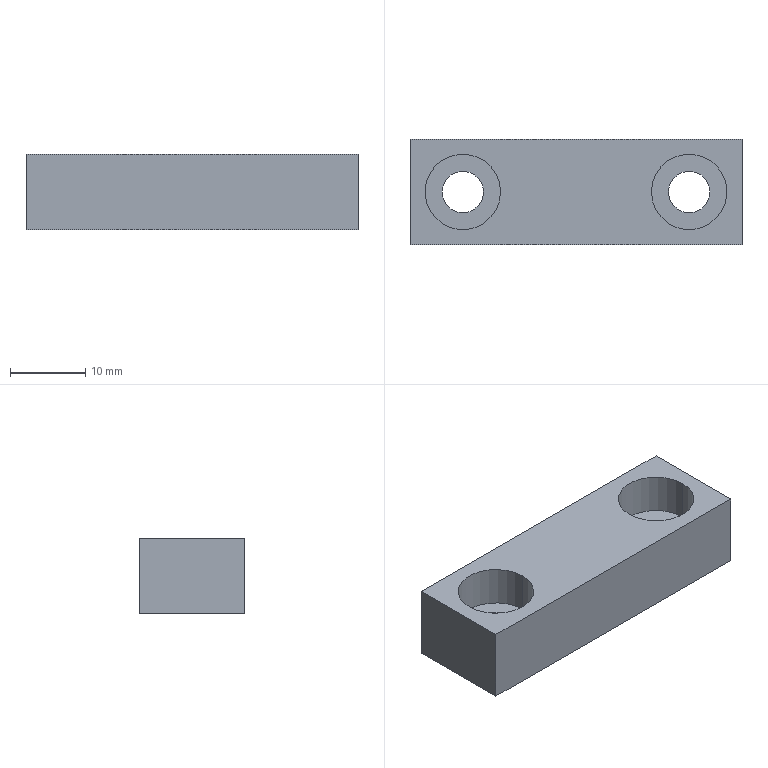Part | STEP file | PN_0061 (stop block) | 1 solid | 16 faces | box 44 x 14 x 10 mm | volume 5093 mm3 | cylinder 8 | plane 8 | commonest cylinder face diameters 5.5 x4 10 x4
STEP:
#1=CARTESIAN_POINT('',(0.,0.,0.));
#2=DIRECTION('',(0.,0.,1.));
#3=DIRECTION('',(1.,0.,0.));
#4=AXIS2_PLACEMENT_3D('',#1,#2,#3);
#5=CARTESIAN_POINT('',(-10.,0.,4.6));
#6=VERTEX_POINT('',#5);
#7=CARTESIAN_POINT('',(-10.,0.,10.));
#8=VERTEX_POINT('',#7);
#9=CARTESIAN_POINT('',(-10.,0.,10.));
#10=DIRECTION('',(0.,0.,1.));
#11=VECTOR('',#10,1.);
#12=LINE('',#9,#11);
#13=CARTESIAN_POINT('',(-15.,0.,10.));
#14=DIRECTION('',(0.,0.,1.));
#15=DIRECTION('',(1.,0.,0.));
#16=AXIS2_PLACEMENT_3D('',#13,#14,#15);
#17=CYLINDRICAL_SURFACE('',#16,5.);
#18=CARTESIAN_POINT('',(6.283,0.));
#19=DIRECTION('',(0.,1.));
#20=VECTOR('',#19,1.);
#21=LINE('',#18,#20);
#22=(GEOMETRIC_REPRESENTATION_CONTEXT(2)PARAMETRIC_REPRESENTATION_CONTEXT()REPRESENTATION_CONTEXT('',''));
#23=DEFINITIONAL_REPRESENTATION('',(#21),#22);
#24=PCURVE('',#17,#23);
#25=CARTESIAN_POINT('',(-15.,0.,10.));
#26=DIRECTION('',(0.,0.,1.));
#27=DIRECTION('',(1.,0.,0.));
#28=AXIS2_PLACEMENT_3D('',#25,#26,#27);
#29=CYLINDRICAL_SURFACE('',#28,5.);
#30=CARTESIAN_POINT('',(0.,0.));
#31=DIRECTION('',(0.,1.));
#32=VECTOR('',#31,1.);
#33=LINE('',#30,#32);
#34=(GEOMETRIC_REPRESENTATION_CONTEXT(2)PARAMETRIC_REPRESENTATION_CONTEXT()REPRESENTATION_CONTEXT('',''));
#35=DEFINITIONAL_REPRESENTATION('',(#33),#34);
#36=PCURVE('',#29,#35);
#37=SURFACE_CURVE('',#12,(#24,#36),.PCURVE_S1.);
#38=EDGE_CURVE('',#6,#8,#37,.T.);
#39=ORIENTED_EDGE('',*,*,#38,.T.);
#40=CARTESIAN_POINT('',(-20.,0.,10.));
#41=VERTEX_POINT('',#40);
#42=CARTESIAN_POINT('',(-15.,0.,10.));
#43=DIRECTION('',(0.,0.,1.));
#44=DIRECTION('',(1.,0.,0.));
#45=AXIS2_PLACEMENT_3D('',#42,#43,#44);
#46=CIRCLE('',#45,5.);
#47=CARTESIAN_POINT('',(0.,0.));
#48=DIRECTION('',(1.,0.));
#49=VECTOR('',#48,1.);
#50=LINE('',#47,#49);
#51=(GEOMETRIC_REPRESENTATION_CONTEXT(2)PARAMETRIC_REPRESENTATION_CONTEXT()REPRESENTATION_CONTEXT('',''));
#52=DEFINITIONAL_REPRESENTATION('',(#50),#51);
#53=PCURVE('',#17,#52);
#54=CARTESIAN_POINT('',(0.,0.,10.));
#55=DIRECTION('',(0.,0.,1.));
#56=DIRECTION('',(1.,0.,0.));
#57=AXIS2_PLACEMENT_3D('',#54,#55,#56);
#58=PLANE('',#57);
#59=CARTESIAN_POINT('',(-15.,0.));
#60=DIRECTION('',(1.,0.));
#61=AXIS2_PLACEMENT_2D('',#59,#60);
#62=CIRCLE('',#61,5.);
#63=(GEOMETRIC_REPRESENTATION_CONTEXT(2)PARAMETRIC_REPRESENTATION_CONTEXT()REPRESENTATION_CONTEXT('',''));
#64=DEFINITIONAL_REPRESENTATION('',(#62),#63);
#65=PCURVE('',#58,#64);
#66=SURFACE_CURVE('',#46,(#53,#65),.PCURVE_S1.);
#67=EDGE_CURVE('',#41,#8,#66,.T.);
#68=ORIENTED_EDGE('',*,*,#67,.F.);
#69=CARTESIAN_POINT('',(-20.,0.,4.6));
#70=VERTEX_POINT('',#69);
#71=CARTESIAN_POINT('',(-20.,0.,10.));
#72=DIRECTION('',(0.,0.,1.));
#73=VECTOR('',#72,1.);
#74=LINE('',#71,#73);
#75=CARTESIAN_POINT('',(3.142,0.));
#76=DIRECTION('',(0.,1.));
#77=VECTOR('',#76,1.);
#78=LINE('',#75,#77);
#79=(GEOMETRIC_REPRESENTATION_CONTEXT(2)PARAMETRIC_REPRESENTATION_CONTEXT()REPRESENTATION_CONTEXT('',''));
#80=DEFINITIONAL_REPRESENTATION('',(#78),#79);
#81=PCURVE('',#17,#80);
#82=CARTESIAN_POINT('',(3.142,0.));
#83=DIRECTION('',(0.,1.));
#84=VECTOR('',#83,1.);
#85=LINE('',#82,#84);
#86=(GEOMETRIC_REPRESENTATION_CONTEXT(2)PARAMETRIC_REPRESENTATION_CONTEXT()REPRESENTATION_CONTEXT('',''));
#87=DEFINITIONAL_REPRESENTATION('',(#85),#86);
#88=PCURVE('',#29,#87);
#89=SURFACE_CURVE('',#74,(#81,#88),.PCURVE_S1.);
#90=EDGE_CURVE('',#70,#41,#89,.T.);
#91=ORIENTED_EDGE('',*,*,#90,.F.);
#92=CARTESIAN_POINT('',(-15.,0.,4.6));
#93=DIRECTION('',(0.,0.,1.));
#94=DIRECTION('',(1.,0.,0.));
#95=AXIS2_PLACEMENT_3D('',#92,#93,#94);
#96=CIRCLE('',#95,5.);
#97=CARTESIAN_POINT('',(0.,-5.4));
#98=DIRECTION('',(1.,0.));
#99=VECTOR('',#98,1.);
#100=LINE('',#97,#99);
#101=(GEOMETRIC_REPRESENTATION_CONTEXT(2)PARAMETRIC_REPRESENTATION_CONTEXT()REPRESENTATION_CONTEXT('',''));
#102=DEFINITIONAL_REPRESENTATION('',(#100),#101);
#103=PCURVE('',#17,#102);
#104=CARTESIAN_POINT('',(-12.25,0.,4.6));
#105=DIRECTION('',(0.,0.,-1.));
#106=DIRECTION('',(-1.,0.,0.));
#107=AXIS2_PLACEMENT_3D('',#104,#105,#106);
#108=PLANE('',#107);
#109=CARTESIAN_POINT('',(-2.25,0.));
#110=CARTESIAN_POINT('',(-2.25,8.66));
#111=CARTESIAN_POINT('',(5.25,4.33));
#112=CARTESIAN_POINT('',(12.75,0.));
#113=CARTESIAN_POINT('',(5.25,-4.33));
#114=CARTESIAN_POINT('',(-2.25,-8.66));
#115=CARTESIAN_POINT('',(-2.25,0.));
#116=(BOUNDED_CURVE()B_SPLINE_CURVE(2,(#109,#110,#111,#112,#113,#114,#115),.UNSPECIFIED.,.T.,.F.)B_SPLINE_CURVE_WITH_KNOTS((1,2,2,2,2,1),(-2.094,0.,2.094,4.189,6.283,8.378),.UNSPECIFIED.)CURVE()GEOMETRIC_REPRESENTATION_ITEM()RATIONAL_B_SPLINE_CURVE((1.,0.5,1.,0.5,1.,0.5,1.))REPRESENTATION_ITEM(''));
#117=(GEOMETRIC_REPRESENTATION_CONTEXT(2)PARAMETRIC_REPRESENTATION_CONTEXT()REPRESENTATION_CONTEXT('',''));
#118=DEFINITIONAL_REPRESENTATION('',(#116),#117);
#119=PCURVE('',#108,#118);
#120=SURFACE_CURVE('',#96,(#103,#119),.PCURVE_S1.);
#121=EDGE_CURVE('',#70,#6,#120,.T.);
#122=ORIENTED_EDGE('',*,*,#121,.T.);
#123=EDGE_LOOP('',(#39,#68,#91,#122));
#124=FACE_BOUND('',#123,.F.);
#125=ADVANCED_FACE('',(#124),#17,.F.);
#126=CARTESIAN_POINT('',(-12.25,0.,0.));
#127=VERTEX_POINT('',#126);
#128=CARTESIAN_POINT('',(-12.25,0.,4.6));
#129=VERTEX_POINT('',#128);
#130=CARTESIAN_POINT('',(-12.25,0.,10.));
#131=DIRECTION('',(0.,0.,1.));
#132=VECTOR('',#131,1.);
#133=LINE('',#130,#132);
#134=CARTESIAN_POINT('',(-15.,0.,10.));
#135=DIRECTION('',(0.,0.,1.));
#136=DIRECTION('',(1.,0.,0.));
#137=AXIS2_PLACEMENT_3D('',#134,#135,#136);
#138=CYLINDRICAL_SURFACE('',#137,2.75);
#139=CARTESIAN_POINT('',(6.283,0.));
#140=DIRECTION('',(0.,1.));
#141=VECTOR('',#140,1.);
#142=LINE('',#139,#141);
#143=(GEOMETRIC_REPRESENTATION_CONTEXT(2)PARAMETRIC_REPRESENTATION_CONTEXT()REPRESENTATION_CONTEXT('',''));
#144=DEFINITIONAL_REPRESENTATION('',(#142),#143);
#145=PCURVE('',#138,#144);
#146=CARTESIAN_POINT('',(-15.,0.,10.));
#147=DIRECTION('',(0.,0.,1.));
#148=DIRECTION('',(1.,0.,0.));
#149=AXIS2_PLACEMENT_3D('',#146,#147,#148);
#150=CYLINDRICAL_SURFACE('',#149,2.75);
#151=CARTESIAN_POINT('',(0.,0.));
#152=DIRECTION('',(0.,1.));
#153=VECTOR('',#152,1.);
#154=LINE('',#151,#153);
#155=(GEOMETRIC_REPRESENTATION_CONTEXT(2)PARAMETRIC_REPRESENTATION_CONTEXT()REPRESENTATION_CONTEXT('',''));
#156=DEFINITIONAL_REPRESENTATION('',(#154),#155);
#157=PCURVE('',#150,#156);
#158=SURFACE_CURVE('',#133,(#145,#157),.PCURVE_S1.);
#159=EDGE_CURVE('',#127,#129,#158,.T.);
#160=ORIENTED_EDGE('',*,*,#159,.T.);
#161=CARTESIAN_POINT('',(-17.75,0.,4.6));
#162=VERTEX_POINT('',#161);
#163=CARTESIAN_POINT('',(-15.,0.,4.6));
#164=DIRECTION('',(0.,0.,1.));
#165=DIRECTION('',(1.,0.,0.));
#166=AXIS2_PLACEMENT_3D('',#163,#164,#165);
#167=CIRCLE('',#166,2.75);
#168=CARTESIAN_POINT('',(0.,-5.4));
#169=DIRECTION('',(1.,0.));
#170=VECTOR('',#169,1.);
#171=LINE('',#168,#170);
#172=(GEOMETRIC_REPRESENTATION_CONTEXT(2)PARAMETRIC_REPRESENTATION_CONTEXT()REPRESENTATION_CONTEXT('',''));
#173=DEFINITIONAL_REPRESENTATION('',(#171),#172);
#174=PCURVE('',#138,#173);
#175=CARTESIAN_POINT('',(0.,0.));
#176=CARTESIAN_POINT('',(0.,4.763));
#177=CARTESIAN_POINT('',(4.125,2.382));
#178=CARTESIAN_POINT('',(8.25,0.));
#179=CARTESIAN_POINT('',(4.125,-2.382));
#180=CARTESIAN_POINT('',(0.,-4.763));
#181=CARTESIAN_POINT('',(0.,0.));
#182=(BOUNDED_CURVE()B_SPLINE_CURVE(2,(#175,#176,#177,#178,#179,#180,#181),.UNSPECIFIED.,.T.,.F.)B_SPLINE_CURVE_WITH_KNOTS((1,2,2,2,2,1),(-2.094,0.,2.094,4.189,6.283,8.378),.UNSPECIFIED.)CURVE()GEOMETRIC_REPRESENTATION_ITEM()RATIONAL_B_SPLINE_CURVE((1.,0.5,1.,0.5,1.,0.5,1.))REPRESENTATION_ITEM(''));
#183=(GEOMETRIC_REPRESENTATION_CONTEXT(2)PARAMETRIC_REPRESENTATION_CONTEXT()REPRESENTATION_CONTEXT('',''));
#184=DEFINITIONAL_REPRESENTATION('',(#182),#183);
#185=PCURVE('',#108,#184);
#186=SURFACE_CURVE('',#167,(#174,#185),.PCURVE_S1.);
#187=EDGE_CURVE('',#162,#129,#186,.T.);
#188=ORIENTED_EDGE('',*,*,#187,.F.);
#189=CARTESIAN_POINT('',(-17.75,0.,0.));
#190=VERTEX_POINT('',#189);
#191=CARTESIAN_POINT('',(-17.75,0.,10.));
#192=DIRECTION('',(0.,0.,1.));
#193=VECTOR('',#192,1.);
#194=LINE('',#191,#193);
#195=CARTESIAN_POINT('',(3.142,0.));
#196=DIRECTION('',(0.,1.));
#197=VECTOR('',#196,1.);
#198=LINE('',#195,#197);
#199=(GEOMETRIC_REPRESENTATION_CONTEXT(2)PARAMETRIC_REPRESENTATION_CONTEXT()REPRESENTATION_CONTEXT('',''));
#200=DEFINITIONAL_REPRESENTATION('',(#198),#199);
#201=PCURVE('',#138,#200);
#202=CARTESIAN_POINT('',(3.142,0.));
#203=DIRECTION('',(0.,1.));
#204=VECTOR('',#203,1.);
#205=LINE('',#202,#204);
#206=(GEOMETRIC_REPRESENTATION_CONTEXT(2)PARAMETRIC_REPRESENTATION_CONTEXT()REPRESENTATION_CONTEXT('',''));
#207=DEFINITIONAL_REPRESENTATION('',(#205),#206);
#208=PCURVE('',#150,#207);
#209=SURFACE_CURVE('',#194,(#201,#208),.PCURVE_S1.);
#210=EDGE_CURVE('',#190,#162,#209,.T.);
#211=ORIENTED_EDGE('',*,*,#210,.F.);
#212=CARTESIAN_POINT('',(-15.,0.,0.));
#213=DIRECTION('',(0.,0.,1.));
#214=DIRECTION('',(1.,0.,0.));
#215=AXIS2_PLACEMENT_3D('',#212,#213,#214);
#216=CIRCLE('',#215,2.75);
#217=CARTESIAN_POINT('',(0.,-10.));
#218=DIRECTION('',(1.,0.));
#219=VECTOR('',#218,1.);
#220=LINE('',#217,#219);
#221=(GEOMETRIC_REPRESENTATION_CONTEXT(2)PARAMETRIC_REPRESENTATION_CONTEXT()REPRESENTATION_CONTEXT('',''));
#222=DEFINITIONAL_REPRESENTATION('',(#220),#221);
#223=PCURVE('',#138,#222);
#224=CARTESIAN_POINT('',(0.,0.,0.));
#225=DIRECTION('',(0.,0.,1.));
#226=DIRECTION('',(1.,0.,0.));
#227=AXIS2_PLACEMENT_3D('',#224,#225,#226);
#228=PLANE('',#227);
#229=CARTESIAN_POINT('',(-15.,0.));
#230=DIRECTION('',(1.,0.));
#231=AXIS2_PLACEMENT_2D('',#229,#230);
#232=CIRCLE('',#231,2.75);
#233=(GEOMETRIC_REPRESENTATION_CONTEXT(2)PARAMETRIC_REPRESENTATION_CONTEXT()REPRESENTATION_CONTEXT('',''));
#234=DEFINITIONAL_REPRESENTATION('',(#232),#233);
#235=PCURVE('',#228,#234);
#236=SURFACE_CURVE('',#216,(#223,#235),.PCURVE_S1.);
#237=EDGE_CURVE('',#190,#127,#236,.T.);
#238=ORIENTED_EDGE('',*,*,#237,.T.);
#239=EDGE_LOOP('',(#160,#188,#211,#238));
#240=FACE_BOUND('',#239,.F.);
#241=ADVANCED_FACE('',(#240),#138,.F.);
#242=CARTESIAN_POINT('',(20.,0.,4.6));
#243=VERTEX_POINT('',#242);
#244=CARTESIAN_POINT('',(20.,0.,10.));
#245=VERTEX_POINT('',#244);
#246=CARTESIAN_POINT('',(20.,0.,10.));
#247=DIRECTION('',(0.,0.,1.));
#248=VECTOR('',#247,1.);
#249=LINE('',#246,#248);
#250=CARTESIAN_POINT('',(15.,0.,10.));
#251=DIRECTION('',(0.,0.,1.));
#252=DIRECTION('',(1.,0.,0.));
#253=AXIS2_PLACEMENT_3D('',#250,#251,#252);
#254=CYLINDRICAL_SURFACE('',#253,5.);
#255=CARTESIAN_POINT('',(6.283,0.));
#256=DIRECTION('',(0.,1.));
#257=VECTOR('',#256,1.);
#258=LINE('',#255,#257);
#259=(GEOMETRIC_REPRESENTATION_CONTEXT(2)PARAMETRIC_REPRESENTATION_CONTEXT()REPRESENTATION_CONTEXT('',''));
#260=DEFINITIONAL_REPRESENTATION('',(#258),#259);
#261=PCURVE('',#254,#260);
#262=CARTESIAN_POINT('',(15.,0.,10.));
#263=DIRECTION('',(0.,0.,1.));
#264=DIRECTION('',(1.,0.,0.));
#265=AXIS2_PLACEMENT_3D('',#262,#263,#264);
#266=CYLINDRICAL_SURFACE('',#265,5.);
#267=CARTESIAN_POINT('',(0.,0.));
#268=DIRECTION('',(0.,1.));
#269=VECTOR('',#268,1.);
#270=LINE('',#267,#269);
#271=(GEOMETRIC_REPRESENTATION_CONTEXT(2)PARAMETRIC_REPRESENTATION_CONTEXT()REPRESENTATION_CONTEXT('',''));
#272=DEFINITIONAL_REPRESENTATION('',(#270),#271);
#273=PCURVE('',#266,#272);
#274=SURFACE_CURVE('',#249,(#261,#273),.PCURVE_S1.);
#275=EDGE_CURVE('',#243,#245,#274,.T.);
#276=ORIENTED_EDGE('',*,*,#275,.T.);
#277=CARTESIAN_POINT('',(10.,0.,10.));
#278=VERTEX_POINT('',#277);
#279=CARTESIAN_POINT('',(15.,0.,10.));
#280=DIRECTION('',(0.,0.,1.));
#281=DIRECTION('',(1.,0.,0.));
#282=AXIS2_PLACEMENT_3D('',#279,#280,#281);
#283=CIRCLE('',#282,5.);
#284=CARTESIAN_POINT('',(0.,0.));
#285=DIRECTION('',(1.,0.));
#286=VECTOR('',#285,1.);
#287=LINE('',#284,#286);
#288=(GEOMETRIC_REPRESENTATION_CONTEXT(2)PARAMETRIC_REPRESENTATION_CONTEXT()REPRESENTATION_CONTEXT('',''));
#289=DEFINITIONAL_REPRESENTATION('',(#287),#288);
#290=PCURVE('',#254,#289);
#291=CARTESIAN_POINT('',(15.,0.));
#292=DIRECTION('',(1.,0.));
#293=AXIS2_PLACEMENT_2D('',#291,#292);
#294=CIRCLE('',#293,5.);
#295=(GEOMETRIC_REPRESENTATION_CONTEXT(2)PARAMETRIC_REPRESENTATION_CONTEXT()REPRESENTATION_CONTEXT('',''));
#296=DEFINITIONAL_REPRESENTATION('',(#294),#295);
#297=PCURVE('',#58,#296);
#298=SURFACE_CURVE('',#283,(#290,#297),.PCURVE_S1.);
#299=EDGE_CURVE('',#278,#245,#298,.T.);
#300=ORIENTED_EDGE('',*,*,#299,.F.);
#301=CARTESIAN_POINT('',(10.,0.,4.6));
#302=VERTEX_POINT('',#301);
#303=CARTESIAN_POINT('',(10.,0.,10.));
#304=DIRECTION('',(0.,0.,1.));
#305=VECTOR('',#304,1.);
#306=LINE('',#303,#305);
#307=CARTESIAN_POINT('',(3.142,0.));
#308=DIRECTION('',(0.,1.));
#309=VECTOR('',#308,1.);
#310=LINE('',#307,#309);
#311=(GEOMETRIC_REPRESENTATION_CONTEXT(2)PARAMETRIC_REPRESENTATION_CONTEXT()REPRESENTATION_CONTEXT('',''));
#312=DEFINITIONAL_REPRESENTATION('',(#310),#311);
#313=PCURVE('',#254,#312);
#314=CARTESIAN_POINT('',(3.142,0.));
#315=DIRECTION('',(0.,1.));
#316=VECTOR('',#315,1.);
#317=LINE('',#314,#316);
#318=(GEOMETRIC_REPRESENTATION_CONTEXT(2)PARAMETRIC_REPRESENTATION_CONTEXT()REPRESENTATION_CONTEXT('',''));
#319=DEFINITIONAL_REPRESENTATION('',(#317),#318);
#320=PCURVE('',#266,#319);
#321=SURFACE_CURVE('',#306,(#313,#320),.PCURVE_S1.);
#322=EDGE_CURVE('',#302,#278,#321,.T.);
#323=ORIENTED_EDGE('',*,*,#322,.F.);
#324=CARTESIAN_POINT('',(15.,0.,4.6));
#325=DIRECTION('',(0.,0.,1.));
#326=DIRECTION('',(1.,0.,0.));
#327=AXIS2_PLACEMENT_3D('',#324,#325,#326);
#328=CIRCLE('',#327,5.);
#329=CARTESIAN_POINT('',(0.,-5.4));
#330=DIRECTION('',(1.,0.));
#331=VECTOR('',#330,1.);
#332=LINE('',#329,#331);
#333=(GEOMETRIC_REPRESENTATION_CONTEXT(2)PARAMETRIC_REPRESENTATION_CONTEXT()REPRESENTATION_CONTEXT('',''));
#334=DEFINITIONAL_REPRESENTATION('',(#332),#333);
#335=PCURVE('',#254,#334);
#336=CARTESIAN_POINT('',(17.75,0.,4.6));
#337=DIRECTION('',(0.,0.,-1.));
#338=DIRECTION('',(-1.,0.,0.));
#339=AXIS2_PLACEMENT_3D('',#336,#337,#338);
#340=PLANE('',#339);
#341=CARTESIAN_POINT('',(-2.25,0.));
#342=CARTESIAN_POINT('',(-2.25,8.66));
#343=CARTESIAN_POINT('',(5.25,4.33));
#344=CARTESIAN_POINT('',(12.75,0.));
#345=CARTESIAN_POINT('',(5.25,-4.33));
#346=CARTESIAN_POINT('',(-2.25,-8.66));
#347=CARTESIAN_POINT('',(-2.25,0.));
#348=(BOUNDED_CURVE()B_SPLINE_CURVE(2,(#341,#342,#343,#344,#345,#346,#347),.UNSPECIFIED.,.T.,.F.)B_SPLINE_CURVE_WITH_KNOTS((1,2,2,2,2,1),(-2.094,0.,2.094,4.189,6.283,8.378),.UNSPECIFIED.)CURVE()GEOMETRIC_REPRESENTATION_ITEM()RATIONAL_B_SPLINE_CURVE((1.,0.5,1.,0.5,1.,0.5,1.))REPRESENTATION_ITEM(''));
#349=(GEOMETRIC_REPRESENTATION_CONTEXT(2)PARAMETRIC_REPRESENTATION_CONTEXT()REPRESENTATION_CONTEXT('',''));
#350=DEFINITIONAL_REPRESENTATION('',(#348),#349);
#351=PCURVE('',#340,#350);
#352=SURFACE_CURVE('',#328,(#335,#351),.PCURVE_S1.);
#353=EDGE_CURVE('',#302,#243,#352,.T.);
#354=ORIENTED_EDGE('',*,*,#353,.T.);
#355=EDGE_LOOP('',(#276,#300,#323,#354));
#356=FACE_BOUND('',#355,.F.);
#357=ADVANCED_FACE('',(#356),#254,.F.);
#358=CARTESIAN_POINT('',(17.75,0.,0.));
#359=VERTEX_POINT('',#358);
#360=CARTESIAN_POINT('',(17.75,0.,4.6));
#361=VERTEX_POINT('',#360);
#362=CARTESIAN_POINT('',(17.75,0.,10.));
#363=DIRECTION('',(0.,0.,1.));
#364=VECTOR('',#363,1.);
#365=LINE('',#362,#364);
#366=CARTESIAN_POINT('',(15.,0.,10.));
#367=DIRECTION('',(0.,0.,1.));
#368=DIRECTION('',(1.,0.,0.));
#369=AXIS2_PLACEMENT_3D('',#366,#367,#368);
#370=CYLINDRICAL_SURFACE('',#369,2.75);
#371=CARTESIAN_POINT('',(6.283,0.));
#372=DIRECTION('',(0.,1.));
#373=VECTOR('',#372,1.);
#374=LINE('',#371,#373);
#375=(GEOMETRIC_REPRESENTATION_CONTEXT(2)PARAMETRIC_REPRESENTATION_CONTEXT()REPRESENTATION_CONTEXT('',''));
#376=DEFINITIONAL_REPRESENTATION('',(#374),#375);
#377=PCURVE('',#370,#376);
#378=CARTESIAN_POINT('',(15.,0.,10.));
#379=DIRECTION('',(0.,0.,1.));
#380=DIRECTION('',(1.,0.,0.));
#381=AXIS2_PLACEMENT_3D('',#378,#379,#380);
#382=CYLINDRICAL_SURFACE('',#381,2.75);
#383=CARTESIAN_POINT('',(0.,0.));
#384=DIRECTION('',(0.,1.));
#385=VECTOR('',#384,1.);
#386=LINE('',#383,#385);
#387=(GEOMETRIC_REPRESENTATION_CONTEXT(2)PARAMETRIC_REPRESENTATION_CONTEXT()REPRESENTATION_CONTEXT('',''));
#388=DEFINITIONAL_REPRESENTATION('',(#386),#387);
#389=PCURVE('',#382,#388);
#390=SURFACE_CURVE('',#365,(#377,#389),.PCURVE_S1.);
#391=EDGE_CURVE('',#359,#361,#390,.T.);
#392=ORIENTED_EDGE('',*,*,#391,.T.);
#393=CARTESIAN_POINT('',(12.25,0.,4.6));
#394=VERTEX_POINT('',#393);
#395=CARTESIAN_POINT('',(15.,0.,4.6));
#396=DIRECTION('',(0.,0.,1.));
#397=DIRECTION('',(1.,0.,0.));
#398=AXIS2_PLACEMENT_3D('',#395,#396,#397);
#399=CIRCLE('',#398,2.75);
#400=CARTESIAN_POINT('',(0.,-5.4));
#401=DIRECTION('',(1.,0.));
#402=VECTOR('',#401,1.);
#403=LINE('',#400,#402);
#404=(GEOMETRIC_REPRESENTATION_CONTEXT(2)PARAMETRIC_REPRESENTATION_CONTEXT()REPRESENTATION_CONTEXT('',''));
#405=DEFINITIONAL_REPRESENTATION('',(#403),#404);
#406=PCURVE('',#370,#405);
#407=CARTESIAN_POINT('',(0.,0.));
#408=CARTESIAN_POINT('',(0.,4.763));
#409=CARTESIAN_POINT('',(4.125,2.382));
#410=CARTESIAN_POINT('',(8.25,0.));
#411=CARTESIAN_POINT('',(4.125,-2.382));
#412=CARTESIAN_POINT('',(0.,-4.763));
#413=CARTESIAN_POINT('',(0.,0.));
#414=(BOUNDED_CURVE()B_SPLINE_CURVE(2,(#407,#408,#409,#410,#411,#412,#413),.UNSPECIFIED.,.T.,.F.)B_SPLINE_CURVE_WITH_KNOTS((1,2,2,2,2,1),(-2.094,0.,2.094,4.189,6.283,8.378),.UNSPECIFIED.)CURVE()GEOMETRIC_REPRESENTATION_ITEM()RATIONAL_B_SPLINE_CURVE((1.,0.5,1.,0.5,1.,0.5,1.))REPRESENTATION_ITEM(''));
#415=(GEOMETRIC_REPRESENTATION_CONTEXT(2)PARAMETRIC_REPRESENTATION_CONTEXT()REPRESENTATION_CONTEXT('',''));
#416=DEFINITIONAL_REPRESENTATION('',(#414),#415);
#417=PCURVE('',#340,#416);
#418=SURFACE_CURVE('',#399,(#406,#417),.PCURVE_S1.);
#419=EDGE_CURVE('',#394,#361,#418,.T.);
#420=ORIENTED_EDGE('',*,*,#419,.F.);
#421=CARTESIAN_POINT('',(12.25,0.,0.));
#422=VERTEX_POINT('',#421);
#423=CARTESIAN_POINT('',(12.25,0.,10.));
#424=DIRECTION('',(0.,0.,1.));
#425=VECTOR('',#424,1.);
#426=LINE('',#423,#425);
#427=CARTESIAN_POINT('',(3.142,0.));
#428=DIRECTION('',(0.,1.));
#429=VECTOR('',#428,1.);
#430=LINE('',#427,#429);
#431=(GEOMETRIC_REPRESENTATION_CONTEXT(2)PARAMETRIC_REPRESENTATION_CONTEXT()REPRESENTATION_CONTEXT('',''));
#432=DEFINITIONAL_REPRESENTATION('',(#430),#431);
#433=PCURVE('',#370,#432);
#434=CARTESIAN_POINT('',(3.142,0.));
#435=DIRECTION('',(0.,1.));
#436=VECTOR('',#435,1.);
#437=LINE('',#434,#436);
#438=(GEOMETRIC_REPRESENTATION_CONTEXT(2)PARAMETRIC_REPRESENTATION_CONTEXT()REPRESENTATION_CONTEXT('',''));
#439=DEFINITIONAL_REPRESENTATION('',(#437),#438);
#440=PCURVE('',#382,#439);
#441=SURFACE_CURVE('',#426,(#433,#440),.PCURVE_S1.);
#442=EDGE_CURVE('',#422,#394,#441,.T.);
#443=ORIENTED_EDGE('',*,*,#442,.F.);
#444=CARTESIAN_POINT('',(15.,0.,0.));
#445=DIRECTION('',(0.,0.,1.));
#446=DIRECTION('',(1.,0.,0.));
#447=AXIS2_PLACEMENT_3D('',#444,#445,#446);
#448=CIRCLE('',#447,2.75);
#449=CARTESIAN_POINT('',(0.,-10.));
#450=DIRECTION('',(1.,0.));
#451=VECTOR('',#450,1.);
#452=LINE('',#449,#451);
#453=(GEOMETRIC_REPRESENTATION_CONTEXT(2)PARAMETRIC_REPRESENTATION_CONTEXT()REPRESENTATION_CONTEXT('',''));
#454=DEFINITIONAL_REPRESENTATION('',(#452),#453);
#455=PCURVE('',#370,#454);
#456=CARTESIAN_POINT('',(15.,0.));
#457=DIRECTION('',(1.,0.));
#458=AXIS2_PLACEMENT_2D('',#456,#457);
#459=CIRCLE('',#458,2.75);
#460=(GEOMETRIC_REPRESENTATION_CONTEXT(2)PARAMETRIC_REPRESENTATION_CONTEXT()REPRESENTATION_CONTEXT('',''));
#461=DEFINITIONAL_REPRESENTATION('',(#459),#460);
#462=PCURVE('',#228,#461);
#463=SURFACE_CURVE('',#448,(#455,#462),.PCURVE_S1.);
#464=EDGE_CURVE('',#422,#359,#463,.T.);
#465=ORIENTED_EDGE('',*,*,#464,.T.);
#466=EDGE_LOOP('',(#392,#420,#443,#465));
#467=FACE_BOUND('',#466,.F.);
#468=ADVANCED_FACE('',(#467),#370,.F.);
#469=CARTESIAN_POINT('',(-22.,7.,0.));
#470=VERTEX_POINT('',#469);
#471=CARTESIAN_POINT('',(-22.,-7.,0.));
#472=VERTEX_POINT('',#471);
#473=CARTESIAN_POINT('',(-22.,-7.,0.));
#474=DIRECTION('',(0.,-1.,0.));
#475=VECTOR('',#474,1.);
#476=LINE('',#473,#475);
#477=CARTESIAN_POINT('',(-22.,-7.,10.));
#478=DIRECTION('',(1.,0.,0.));
#479=DIRECTION('',(0.,0.,-1.));
#480=AXIS2_PLACEMENT_3D('',#477,#478,#479);
#481=PLANE('',#480);
#482=CARTESIAN_POINT('',(10.,0.));
#483=DIRECTION('',(0.,-1.));
#484=VECTOR('',#483,1.);
#485=LINE('',#482,#484);
#486=(GEOMETRIC_REPRESENTATION_CONTEXT(2)PARAMETRIC_REPRESENTATION_CONTEXT()REPRESENTATION_CONTEXT('',''));
#487=DEFINITIONAL_REPRESENTATION('',(#485),#486);
#488=PCURVE('',#481,#487);
#489=CARTESIAN_POINT('',(-22.,-7.));
#490=DIRECTION('',(0.,-1.));
#491=VECTOR('',#490,1.);
#492=LINE('',#489,#491);
#493=(GEOMETRIC_REPRESENTATION_CONTEXT(2)PARAMETRIC_REPRESENTATION_CONTEXT()REPRESENTATION_CONTEXT('',''));
#494=DEFINITIONAL_REPRESENTATION('',(#492),#493);
#495=PCURVE('',#228,#494);
#496=SURFACE_CURVE('',#476,(#488,#495),.PCURVE_S1.);
#497=EDGE_CURVE('',#470,#472,#496,.T.);
#498=ORIENTED_EDGE('',*,*,#497,.T.);
#499=CARTESIAN_POINT('',(-22.,-7.,10.));
#500=VERTEX_POINT('',#499);
#501=CARTESIAN_POINT('',(-22.,-7.,10.));
#502=DIRECTION('',(0.,0.,-1.));
#503=VECTOR('',#502,1.);
#504=LINE('',#501,#503);
#505=CARTESIAN_POINT('',(0.,0.));
#506=DIRECTION('',(1.,0.));
#507=VECTOR('',#506,1.);
#508=LINE('',#505,#507);
#509=(GEOMETRIC_REPRESENTATION_CONTEXT(2)PARAMETRIC_REPRESENTATION_CONTEXT()REPRESENTATION_CONTEXT('',''));
#510=DEFINITIONAL_REPRESENTATION('',(#508),#509);
#511=PCURVE('',#481,#510);
#512=CARTESIAN_POINT('',(22.,-7.,10.));
#513=DIRECTION('',(0.,1.,0.));
#514=DIRECTION('',(-1.,0.,0.));
#515=AXIS2_PLACEMENT_3D('',#512,#513,#514);
#516=PLANE('',#515);
#517=CARTESIAN_POINT('',(44.,0.));
#518=DIRECTION('',(0.,-1.));
#519=VECTOR('',#518,1.);
#520=LINE('',#517,#519);
#521=(GEOMETRIC_REPRESENTATION_CONTEXT(2)PARAMETRIC_REPRESENTATION_CONTEXT()REPRESENTATION_CONTEXT('',''));
#522=DEFINITIONAL_REPRESENTATION('',(#520),#521);
#523=PCURVE('',#516,#522);
#524=SURFACE_CURVE('',#504,(#511,#523),.PCURVE_S1.);
#525=EDGE_CURVE('',#500,#472,#524,.T.);
#526=ORIENTED_EDGE('',*,*,#525,.F.);
#527=CARTESIAN_POINT('',(-22.,7.,10.));
#528=VERTEX_POINT('',#527);
#529=CARTESIAN_POINT('',(-22.,-7.,10.));
#530=DIRECTION('',(0.,-1.,0.));
#531=VECTOR('',#530,1.);
#532=LINE('',#529,#531);
#533=CARTESIAN_POINT('',(0.,0.));
#534=DIRECTION('',(0.,-1.));
#535=VECTOR('',#534,1.);
#536=LINE('',#533,#535);
#537=(GEOMETRIC_REPRESENTATION_CONTEXT(2)PARAMETRIC_REPRESENTATION_CONTEXT()REPRESENTATION_CONTEXT('',''));
#538=DEFINITIONAL_REPRESENTATION('',(#536),#537);
#539=PCURVE('',#481,#538);
#540=CARTESIAN_POINT('',(-22.,-7.));
#541=DIRECTION('',(0.,-1.));
#542=VECTOR('',#541,1.);
#543=LINE('',#540,#542);
#544=(GEOMETRIC_REPRESENTATION_CONTEXT(2)PARAMETRIC_REPRESENTATION_CONTEXT()REPRESENTATION_CONTEXT('',''));
#545=DEFINITIONAL_REPRESENTATION('',(#543),#544);
#546=PCURVE('',#58,#545);
#547=SURFACE_CURVE('',#532,(#539,#546),.PCURVE_S1.);
#548=EDGE_CURVE('',#528,#500,#547,.T.);
#549=ORIENTED_EDGE('',*,*,#548,.F.);
#550=CARTESIAN_POINT('',(-22.,7.,10.));
#551=DIRECTION('',(0.,0.,-1.));
#552=VECTOR('',#551,1.);
#553=LINE('',#550,#552);
#554=CARTESIAN_POINT('',(0.,14.));
#555=DIRECTION('',(1.,0.));
#556=VECTOR('',#555,1.);
#557=LINE('',#554,#556);
#558=(GEOMETRIC_REPRESENTATION_CONTEXT(2)PARAMETRIC_REPRESENTATION_CONTEXT()REPRESENTATION_CONTEXT('',''));
#559=DEFINITIONAL_REPRESENTATION('',(#557),#558);
#560=PCURVE('',#481,#559);
#561=CARTESIAN_POINT('',(22.,7.,10.));
#562=DIRECTION('',(0.,-1.,0.));
#563=DIRECTION('',(1.,0.,0.));
#564=AXIS2_PLACEMENT_3D('',#561,#562,#563);
#565=PLANE('',#564);
#566=CARTESIAN_POINT('',(-44.,0.));
#567=DIRECTION('',(0.,-1.));
#568=VECTOR('',#567,1.);
#569=LINE('',#566,#568);
#570=(GEOMETRIC_REPRESENTATION_CONTEXT(2)PARAMETRIC_REPRESENTATION_CONTEXT()REPRESENTATION_CONTEXT('',''));
#571=DEFINITIONAL_REPRESENTATION('',(#569),#570);
#572=PCURVE('',#565,#571);
#573=SURFACE_CURVE('',#553,(#560,#572),.PCURVE_S1.);
#574=EDGE_CURVE('',#528,#470,#573,.T.);
#575=ORIENTED_EDGE('',*,*,#574,.T.);
#576=EDGE_LOOP('',(#498,#526,#549,#575));
#577=FACE_BOUND('',#576,.T.);
#578=ADVANCED_FACE('',(#577),#481,.F.);
#579=CARTESIAN_POINT('',(22.,-7.,0.));
#580=VERTEX_POINT('',#579);
#581=CARTESIAN_POINT('',(22.,-7.,0.));
#582=DIRECTION('',(1.,0.,0.));
#583=VECTOR('',#582,1.);
#584=LINE('',#581,#583);
#585=CARTESIAN_POINT('',(0.,-10.));
#586=DIRECTION('',(-1.,0.));
#587=VECTOR('',#586,1.);
#588=LINE('',#585,#587);
#589=(GEOMETRIC_REPRESENTATION_CONTEXT(2)PARAMETRIC_REPRESENTATION_CONTEXT()REPRESENTATION_CONTEXT('',''));
#590=DEFINITIONAL_REPRESENTATION('',(#588),#589);
#591=PCURVE('',#516,#590);
#592=CARTESIAN_POINT('',(22.,-7.));
#593=DIRECTION('',(1.,0.));
#594=VECTOR('',#593,1.);
#595=LINE('',#592,#594);
#596=(GEOMETRIC_REPRESENTATION_CONTEXT(2)PARAMETRIC_REPRESENTATION_CONTEXT()REPRESENTATION_CONTEXT('',''));
#597=DEFINITIONAL_REPRESENTATION('',(#595),#596);
#598=PCURVE('',#228,#597);
#599=SURFACE_CURVE('',#584,(#591,#598),.PCURVE_S1.);
#600=EDGE_CURVE('',#472,#580,#599,.T.);
#601=ORIENTED_EDGE('',*,*,#600,.T.);
#602=CARTESIAN_POINT('',(22.,-7.,10.));
#603=VERTEX_POINT('',#602);
#604=CARTESIAN_POINT('',(22.,-7.,10.));
#605=DIRECTION('',(0.,0.,-1.));
#606=VECTOR('',#605,1.);
#607=LINE('',#604,#606);
#608=CARTESIAN_POINT('',(0.,0.));
#609=DIRECTION('',(0.,-1.));
#610=VECTOR('',#609,1.);
#611=LINE('',#608,#610);
#612=(GEOMETRIC_REPRESENTATION_CONTEXT(2)PARAMETRIC_REPRESENTATION_CONTEXT()REPRESENTATION_CONTEXT('',''));
#613=DEFINITIONAL_REPRESENTATION('',(#611),#612);
#614=PCURVE('',#516,#613);
#615=CARTESIAN_POINT('',(22.,-7.,10.));
#616=DIRECTION('',(-1.,0.,0.));
#617=DIRECTION('',(0.,0.,1.));
#618=AXIS2_PLACEMENT_3D('',#615,#616,#617);
#619=PLANE('',#618);
#620=CARTESIAN_POINT('',(0.,0.));
#621=DIRECTION('',(-1.,0.));
#622=VECTOR('',#621,1.);
#623=LINE('',#620,#622);
#624=(GEOMETRIC_REPRESENTATION_CONTEXT(2)PARAMETRIC_REPRESENTATION_CONTEXT()REPRESENTATION_CONTEXT('',''));
#625=DEFINITIONAL_REPRESENTATION('',(#623),#624);
#626=PCURVE('',#619,#625);
#627=SURFACE_CURVE('',#607,(#614,#626),.PCURVE_S1.);
#628=EDGE_CURVE('',#603,#580,#627,.T.);
#629=ORIENTED_EDGE('',*,*,#628,.F.);
#630=CARTESIAN_POINT('',(22.,-7.,10.));
#631=DIRECTION('',(1.,0.,0.));
#632=VECTOR('',#631,1.);
#633=LINE('',#630,#632);
#634=CARTESIAN_POINT('',(0.,0.));
#635=DIRECTION('',(-1.,0.));
#636=VECTOR('',#635,1.);
#637=LINE('',#634,#636);
#638=(GEOMETRIC_REPRESENTATION_CONTEXT(2)PARAMETRIC_REPRESENTATION_CONTEXT()REPRESENTATION_CONTEXT('',''));
#639=DEFINITIONAL_REPRESENTATION('',(#637),#638);
#640=PCURVE('',#516,#639);
#641=CARTESIAN_POINT('',(22.,-7.));
#642=DIRECTION('',(1.,0.));
#643=VECTOR('',#642,1.);
#644=LINE('',#641,#643);
#645=(GEOMETRIC_REPRESENTATION_CONTEXT(2)PARAMETRIC_REPRESENTATION_CONTEXT()REPRESENTATION_CONTEXT('',''));
#646=DEFINITIONAL_REPRESENTATION('',(#644),#645);
#647=PCURVE('',#58,#646);
#648=SURFACE_CURVE('',#633,(#640,#647),.PCURVE_S1.);
#649=EDGE_CURVE('',#500,#603,#648,.T.);
#650=ORIENTED_EDGE('',*,*,#649,.F.);
#651=ORIENTED_EDGE('',*,*,#525,.T.);
#652=EDGE_LOOP('',(#601,#629,#650,#651));
#653=FACE_BOUND('',#652,.T.);
#654=ADVANCED_FACE('',(#653),#516,.F.);
#655=CARTESIAN_POINT('',(22.,7.,0.));
#656=VERTEX_POINT('',#655);
#657=CARTESIAN_POINT('',(22.,-7.,0.));
#658=DIRECTION('',(0.,1.,0.));
#659=VECTOR('',#658,1.);
#660=LINE('',#657,#659);
#661=CARTESIAN_POINT('',(-10.,0.));
#662=DIRECTION('',(0.,1.));
#663=VECTOR('',#662,1.);
#664=LINE('',#661,#663);
#665=(GEOMETRIC_REPRESENTATION_CONTEXT(2)PARAMETRIC_REPRESENTATION_CONTEXT()REPRESENTATION_CONTEXT('',''));
#666=DEFINITIONAL_REPRESENTATION('',(#664),#665);
#667=PCURVE('',#619,#666);
#668=CARTESIAN_POINT('',(22.,-7.));
#669=DIRECTION('',(0.,1.));
#670=VECTOR('',#669,1.);
#671=LINE('',#668,#670);
#672=(GEOMETRIC_REPRESENTATION_CONTEXT(2)PARAMETRIC_REPRESENTATION_CONTEXT()REPRESENTATION_CONTEXT('',''));
#673=DEFINITIONAL_REPRESENTATION('',(#671),#672);
#674=PCURVE('',#228,#673);
#675=SURFACE_CURVE('',#660,(#667,#674),.PCURVE_S1.);
#676=EDGE_CURVE('',#580,#656,#675,.T.);
#677=ORIENTED_EDGE('',*,*,#676,.T.);
#678=CARTESIAN_POINT('',(22.,7.,10.));
#679=VERTEX_POINT('',#678);
#680=CARTESIAN_POINT('',(22.,7.,10.));
#681=DIRECTION('',(0.,0.,-1.));
#682=VECTOR('',#681,1.);
#683=LINE('',#680,#682);
#684=CARTESIAN_POINT('',(0.,14.));
#685=DIRECTION('',(-1.,0.));
#686=VECTOR('',#685,1.);
#687=LINE('',#684,#686);
#688=(GEOMETRIC_REPRESENTATION_CONTEXT(2)PARAMETRIC_REPRESENTATION_CONTEXT()REPRESENTATION_CONTEXT('',''));
#689=DEFINITIONAL_REPRESENTATION('',(#687),#688);
#690=PCURVE('',#619,#689);
#691=CARTESIAN_POINT('',(0.,0.));
#692=DIRECTION('',(0.,-1.));
#693=VECTOR('',#692,1.);
#694=LINE('',#691,#693);
#695=(GEOMETRIC_REPRESENTATION_CONTEXT(2)PARAMETRIC_REPRESENTATION_CONTEXT()REPRESENTATION_CONTEXT('',''));
#696=DEFINITIONAL_REPRESENTATION('',(#694),#695);
#697=PCURVE('',#565,#696);
#698=SURFACE_CURVE('',#683,(#690,#697),.PCURVE_S1.);
#699=EDGE_CURVE('',#679,#656,#698,.T.);
#700=ORIENTED_EDGE('',*,*,#699,.F.);
#701=CARTESIAN_POINT('',(22.,-7.,10.));
#702=DIRECTION('',(0.,1.,0.));
#703=VECTOR('',#702,1.);
#704=LINE('',#701,#703);
#705=CARTESIAN_POINT('',(0.,0.));
#706=DIRECTION('',(0.,1.));
#707=VECTOR('',#706,1.);
#708=LINE('',#705,#707);
#709=(GEOMETRIC_REPRESENTATION_CONTEXT(2)PARAMETRIC_REPRESENTATION_CONTEXT()REPRESENTATION_CONTEXT('',''));
#710=DEFINITIONAL_REPRESENTATION('',(#708),#709);
#711=PCURVE('',#619,#710);
#712=CARTESIAN_POINT('',(22.,-7.));
#713=DIRECTION('',(0.,1.));
#714=VECTOR('',#713,1.);
#715=LINE('',#712,#714);
#716=(GEOMETRIC_REPRESENTATION_CONTEXT(2)PARAMETRIC_REPRESENTATION_CONTEXT()REPRESENTATION_CONTEXT('',''));
#717=DEFINITIONAL_REPRESENTATION('',(#715),#716);
#718=PCURVE('',#58,#717);
#719=SURFACE_CURVE('',#704,(#711,#718),.PCURVE_S1.);
#720=EDGE_CURVE('',#603,#679,#719,.T.);
#721=ORIENTED_EDGE('',*,*,#720,.F.);
#722=ORIENTED_EDGE('',*,*,#628,.T.);
#723=EDGE_LOOP('',(#677,#700,#721,#722));
#724=FACE_BOUND('',#723,.T.);
#725=ADVANCED_FACE('',(#724),#619,.F.);
#726=CARTESIAN_POINT('',(22.,7.,0.));
#727=DIRECTION('',(-1.,0.,0.));
#728=VECTOR('',#727,1.);
#729=LINE('',#726,#728);
#730=CARTESIAN_POINT('',(0.,-10.));
#731=DIRECTION('',(-1.,0.));
#732=VECTOR('',#731,1.);
#733=LINE('',#730,#732);
#734=(GEOMETRIC_REPRESENTATION_CONTEXT(2)PARAMETRIC_REPRESENTATION_CONTEXT()REPRESENTATION_CONTEXT('',''));
#735=DEFINITIONAL_REPRESENTATION('',(#733),#734);
#736=PCURVE('',#565,#735);
#737=CARTESIAN_POINT('',(22.,7.));
#738=DIRECTION('',(-1.,0.));
#739=VECTOR('',#738,1.);
#740=LINE('',#737,#739);
#741=(GEOMETRIC_REPRESENTATION_CONTEXT(2)PARAMETRIC_REPRESENTATION_CONTEXT()REPRESENTATION_CONTEXT('',''));
#742=DEFINITIONAL_REPRESENTATION('',(#740),#741);
#743=PCURVE('',#228,#742);
#744=SURFACE_CURVE('',#729,(#736,#743),.PCURVE_S1.);
#745=EDGE_CURVE('',#656,#470,#744,.T.);
#746=ORIENTED_EDGE('',*,*,#745,.T.);
#747=ORIENTED_EDGE('',*,*,#574,.F.);
#748=CARTESIAN_POINT('',(22.,7.,10.));
#749=DIRECTION('',(-1.,0.,0.));
#750=VECTOR('',#749,1.);
#751=LINE('',#748,#750);
#752=CARTESIAN_POINT('',(0.,0.));
#753=DIRECTION('',(-1.,0.));
#754=VECTOR('',#753,1.);
#755=LINE('',#752,#754);
#756=(GEOMETRIC_REPRESENTATION_CONTEXT(2)PARAMETRIC_REPRESENTATION_CONTEXT()REPRESENTATION_CONTEXT('',''));
#757=DEFINITIONAL_REPRESENTATION('',(#755),#756);
#758=PCURVE('',#565,#757);
#759=CARTESIAN_POINT('',(22.,7.));
#760=DIRECTION('',(-1.,0.));
#761=VECTOR('',#760,1.);
#762=LINE('',#759,#761);
#763=(GEOMETRIC_REPRESENTATION_CONTEXT(2)PARAMETRIC_REPRESENTATION_CONTEXT()REPRESENTATION_CONTEXT('',''));
#764=DEFINITIONAL_REPRESENTATION('',(#762),#763);
#765=PCURVE('',#58,#764);
#766=SURFACE_CURVE('',#751,(#758,#765),.PCURVE_S1.);
#767=EDGE_CURVE('',#679,#528,#766,.T.);
#768=ORIENTED_EDGE('',*,*,#767,.F.);
#769=ORIENTED_EDGE('',*,*,#699,.T.);
#770=EDGE_LOOP('',(#746,#747,#768,#769));
#771=FACE_BOUND('',#770,.T.);
#772=ADVANCED_FACE('',(#771),#565,.F.);
#773=CARTESIAN_POINT('',(-15.,0.,10.));
#774=DIRECTION('',(0.,0.,1.));
#775=DIRECTION('',(1.,0.,0.));
#776=AXIS2_PLACEMENT_3D('',#773,#774,#775);
#777=CIRCLE('',#776,5.);
#778=CARTESIAN_POINT('',(-15.,0.));
#779=DIRECTION('',(1.,0.));
#780=AXIS2_PLACEMENT_2D('',#778,#779);
#781=CIRCLE('',#780,5.);
#782=(GEOMETRIC_REPRESENTATION_CONTEXT(2)PARAMETRIC_REPRESENTATION_CONTEXT()REPRESENTATION_CONTEXT('',''));
#783=DEFINITIONAL_REPRESENTATION('',(#781),#782);
#784=PCURVE('',#58,#783);
#785=CARTESIAN_POINT('',(0.,0.));
#786=DIRECTION('',(1.,0.));
#787=VECTOR('',#786,1.);
#788=LINE('',#785,#787);
#789=(GEOMETRIC_REPRESENTATION_CONTEXT(2)PARAMETRIC_REPRESENTATION_CONTEXT()REPRESENTATION_CONTEXT('',''));
#790=DEFINITIONAL_REPRESENTATION('',(#788),#789);
#791=PCURVE('',#29,#790);
#792=SURFACE_CURVE('',#777,(#784,#791),.PCURVE_S1.);
#793=EDGE_CURVE('',#8,#41,#792,.T.);
#794=ORIENTED_EDGE('',*,*,#793,.F.);
#795=ORIENTED_EDGE('',*,*,#67,.F.);
#796=EDGE_LOOP('',(#794,#795));
#797=FACE_BOUND('',#796,.T.);
#798=CARTESIAN_POINT('',(15.,0.,10.));
#799=DIRECTION('',(0.,0.,1.));
#800=DIRECTION('',(1.,0.,0.));
#801=AXIS2_PLACEMENT_3D('',#798,#799,#800);
#802=CIRCLE('',#801,5.);
#803=CARTESIAN_POINT('',(15.,0.));
#804=DIRECTION('',(1.,0.));
#805=AXIS2_PLACEMENT_2D('',#803,#804);
#806=CIRCLE('',#805,5.);
#807=(GEOMETRIC_REPRESENTATION_CONTEXT(2)PARAMETRIC_REPRESENTATION_CONTEXT()REPRESENTATION_CONTEXT('',''));
#808=DEFINITIONAL_REPRESENTATION('',(#806),#807);
#809=PCURVE('',#58,#808);
#810=CARTESIAN_POINT('',(0.,0.));
#811=DIRECTION('',(1.,0.));
#812=VECTOR('',#811,1.);
#813=LINE('',#810,#812);
#814=(GEOMETRIC_REPRESENTATION_CONTEXT(2)PARAMETRIC_REPRESENTATION_CONTEXT()REPRESENTATION_CONTEXT('',''));
#815=DEFINITIONAL_REPRESENTATION('',(#813),#814);
#816=PCURVE('',#266,#815);
#817=SURFACE_CURVE('',#802,(#809,#816),.PCURVE_S1.);
#818=EDGE_CURVE('',#245,#278,#817,.T.);
#819=ORIENTED_EDGE('',*,*,#818,.F.);
#820=ORIENTED_EDGE('',*,*,#299,.F.);
#821=EDGE_LOOP('',(#819,#820));
#822=FACE_BOUND('',#821,.T.);
#823=ORIENTED_EDGE('',*,*,#548,.T.);
#824=ORIENTED_EDGE('',*,*,#649,.T.);
#825=ORIENTED_EDGE('',*,*,#720,.T.);
#826=ORIENTED_EDGE('',*,*,#767,.T.);
#827=EDGE_LOOP('',(#823,#824,#825,#826));
#828=FACE_BOUND('',#827,.T.);
#829=ADVANCED_FACE('',(#797,#822,#828),#58,.T.);
#830=CARTESIAN_POINT('',(-15.,0.,0.));
#831=DIRECTION('',(0.,0.,1.));
#832=DIRECTION('',(1.,0.,0.));
#833=AXIS2_PLACEMENT_3D('',#830,#831,#832);
#834=CIRCLE('',#833,2.75);
#835=CARTESIAN_POINT('',(-15.,0.));
#836=DIRECTION('',(1.,0.));
#837=AXIS2_PLACEMENT_2D('',#835,#836);
#838=CIRCLE('',#837,2.75);
#839=(GEOMETRIC_REPRESENTATION_CONTEXT(2)PARAMETRIC_REPRESENTATION_CONTEXT()REPRESENTATION_CONTEXT('',''));
#840=DEFINITIONAL_REPRESENTATION('',(#838),#839);
#841=PCURVE('',#228,#840);
#842=CARTESIAN_POINT('',(0.,-10.));
#843=DIRECTION('',(1.,0.));
#844=VECTOR('',#843,1.);
#845=LINE('',#842,#844);
#846=(GEOMETRIC_REPRESENTATION_CONTEXT(2)PARAMETRIC_REPRESENTATION_CONTEXT()REPRESENTATION_CONTEXT('',''));
#847=DEFINITIONAL_REPRESENTATION('',(#845),#846);
#848=PCURVE('',#150,#847);
#849=SURFACE_CURVE('',#834,(#841,#848),.PCURVE_S1.);
#850=EDGE_CURVE('',#127,#190,#849,.T.);
#851=ORIENTED_EDGE('',*,*,#850,.T.);
#852=ORIENTED_EDGE('',*,*,#237,.T.);
#853=EDGE_LOOP('',(#851,#852));
#854=FACE_BOUND('',#853,.T.);
#855=CARTESIAN_POINT('',(15.,0.,0.));
#856=DIRECTION('',(0.,0.,1.));
#857=DIRECTION('',(1.,0.,0.));
#858=AXIS2_PLACEMENT_3D('',#855,#856,#857);
#859=CIRCLE('',#858,2.75);
#860=CARTESIAN_POINT('',(15.,0.));
#861=DIRECTION('',(1.,0.));
#862=AXIS2_PLACEMENT_2D('',#860,#861);
#863=CIRCLE('',#862,2.75);
#864=(GEOMETRIC_REPRESENTATION_CONTEXT(2)PARAMETRIC_REPRESENTATION_CONTEXT()REPRESENTATION_CONTEXT('',''));
#865=DEFINITIONAL_REPRESENTATION('',(#863),#864);
#866=PCURVE('',#228,#865);
#867=CARTESIAN_POINT('',(0.,-10.));
#868=DIRECTION('',(1.,0.));
#869=VECTOR('',#868,1.);
#870=LINE('',#867,#869);
#871=(GEOMETRIC_REPRESENTATION_CONTEXT(2)PARAMETRIC_REPRESENTATION_CONTEXT()REPRESENTATION_CONTEXT('',''));
#872=DEFINITIONAL_REPRESENTATION('',(#870),#871);
#873=PCURVE('',#382,#872);
#874=SURFACE_CURVE('',#859,(#866,#873),.PCURVE_S1.);
#875=EDGE_CURVE('',#359,#422,#874,.T.);
#876=ORIENTED_EDGE('',*,*,#875,.T.);
#877=ORIENTED_EDGE('',*,*,#464,.T.);
#878=EDGE_LOOP('',(#876,#877));
#879=FACE_BOUND('',#878,.T.);
#880=ORIENTED_EDGE('',*,*,#497,.F.);
#881=ORIENTED_EDGE('',*,*,#745,.F.);
#882=ORIENTED_EDGE('',*,*,#676,.F.);
#883=ORIENTED_EDGE('',*,*,#600,.F.);
#884=EDGE_LOOP('',(#880,#881,#882,#883));
#885=FACE_BOUND('',#884,.T.);
#886=ADVANCED_FACE('',(#854,#879,#885),#228,.F.);
#887=CARTESIAN_POINT('',(15.,0.,4.6));
#888=DIRECTION('',(0.,0.,1.));
#889=DIRECTION('',(1.,0.,0.));
#890=AXIS2_PLACEMENT_3D('',#887,#888,#889);
#891=CIRCLE('',#890,2.75);
#892=CARTESIAN_POINT('',(0.,-5.4));
#893=DIRECTION('',(1.,0.));
#894=VECTOR('',#893,1.);
#895=LINE('',#892,#894);
#896=(GEOMETRIC_REPRESENTATION_CONTEXT(2)PARAMETRIC_REPRESENTATION_CONTEXT()REPRESENTATION_CONTEXT('',''));
#897=DEFINITIONAL_REPRESENTATION('',(#895),#896);
#898=PCURVE('',#382,#897);
#899=CARTESIAN_POINT('',(0.,0.));
#900=CARTESIAN_POINT('',(0.,4.763));
#901=CARTESIAN_POINT('',(4.125,2.382));
#902=CARTESIAN_POINT('',(8.25,0.));
#903=CARTESIAN_POINT('',(4.125,-2.382));
#904=CARTESIAN_POINT('',(0.,-4.763));
#905=CARTESIAN_POINT('',(0.,0.));
#906=(BOUNDED_CURVE()B_SPLINE_CURVE(2,(#899,#900,#901,#902,#903,#904,#905),.UNSPECIFIED.,.T.,.F.)B_SPLINE_CURVE_WITH_KNOTS((1,2,2,2,2,1),(-2.094,0.,2.094,4.189,6.283,8.378),.UNSPECIFIED.)CURVE()GEOMETRIC_REPRESENTATION_ITEM()RATIONAL_B_SPLINE_CURVE((1.,0.5,1.,0.5,1.,0.5,1.))REPRESENTATION_ITEM(''));
#907=(GEOMETRIC_REPRESENTATION_CONTEXT(2)PARAMETRIC_REPRESENTATION_CONTEXT()REPRESENTATION_CONTEXT('',''));
#908=DEFINITIONAL_REPRESENTATION('',(#906),#907);
#909=PCURVE('',#340,#908);
#910=SURFACE_CURVE('',#891,(#898,#909),.PCURVE_S1.);
#911=EDGE_CURVE('',#361,#394,#910,.T.);
#912=ORIENTED_EDGE('',*,*,#911,.F.);
#913=ORIENTED_EDGE('',*,*,#391,.F.);
#914=ORIENTED_EDGE('',*,*,#875,.T.);
#915=ORIENTED_EDGE('',*,*,#442,.T.);
#916=EDGE_LOOP('',(#912,#913,#914,#915));
#917=FACE_BOUND('',#916,.F.);
#918=ADVANCED_FACE('',(#917),#382,.F.);
#919=ORIENTED_EDGE('',*,*,#911,.F.);
#920=ORIENTED_EDGE('',*,*,#419,.F.);
#921=EDGE_LOOP('',(#919,#920));
#922=FACE_BOUND('',#921,.T.);
#923=CARTESIAN_POINT('',(15.,0.,4.6));
#924=DIRECTION('',(0.,0.,1.));
#925=DIRECTION('',(1.,0.,0.));
#926=AXIS2_PLACEMENT_3D('',#923,#924,#925);
#927=CIRCLE('',#926,5.);
#928=CARTESIAN_POINT('',(-2.25,0.));
#929=CARTESIAN_POINT('',(-2.25,8.66));
#930=CARTESIAN_POINT('',(5.25,4.33));
#931=CARTESIAN_POINT('',(12.75,0.));
#932=CARTESIAN_POINT('',(5.25,-4.33));
#933=CARTESIAN_POINT('',(-2.25,-8.66));
#934=CARTESIAN_POINT('',(-2.25,0.));
#935=(BOUNDED_CURVE()B_SPLINE_CURVE(2,(#928,#929,#930,#931,#932,#933,#934),.UNSPECIFIED.,.T.,.F.)B_SPLINE_CURVE_WITH_KNOTS((1,2,2,2,2,1),(-2.094,0.,2.094,4.189,6.283,8.378),.UNSPECIFIED.)CURVE()GEOMETRIC_REPRESENTATION_ITEM()RATIONAL_B_SPLINE_CURVE((1.,0.5,1.,0.5,1.,0.5,1.))REPRESENTATION_ITEM(''));
#936=(GEOMETRIC_REPRESENTATION_CONTEXT(2)PARAMETRIC_REPRESENTATION_CONTEXT()REPRESENTATION_CONTEXT('',''));
#937=DEFINITIONAL_REPRESENTATION('',(#935),#936);
#938=PCURVE('',#340,#937);
#939=CARTESIAN_POINT('',(0.,-5.4));
#940=DIRECTION('',(1.,0.));
#941=VECTOR('',#940,1.);
#942=LINE('',#939,#941);
#943=(GEOMETRIC_REPRESENTATION_CONTEXT(2)PARAMETRIC_REPRESENTATION_CONTEXT()REPRESENTATION_CONTEXT('',''));
#944=DEFINITIONAL_REPRESENTATION('',(#942),#943);
#945=PCURVE('',#266,#944);
#946=SURFACE_CURVE('',#927,(#938,#945),.PCURVE_S1.);
#947=EDGE_CURVE('',#243,#302,#946,.T.);
#948=ORIENTED_EDGE('',*,*,#947,.T.);
#949=ORIENTED_EDGE('',*,*,#353,.T.);
#950=EDGE_LOOP('',(#948,#949));
#951=FACE_BOUND('',#950,.T.);
#952=ADVANCED_FACE('',(#922,#951),#340,.F.);
#953=ORIENTED_EDGE('',*,*,#818,.F.);
#954=ORIENTED_EDGE('',*,*,#275,.F.);
#955=ORIENTED_EDGE('',*,*,#947,.T.);
#956=ORIENTED_EDGE('',*,*,#322,.T.);
#957=EDGE_LOOP('',(#953,#954,#955,#956));
#958=FACE_BOUND('',#957,.F.);
#959=ADVANCED_FACE('',(#958),#266,.F.);
#960=CARTESIAN_POINT('',(-15.,0.,4.6));
#961=DIRECTION('',(0.,0.,1.));
#962=DIRECTION('',(1.,0.,0.));
#963=AXIS2_PLACEMENT_3D('',#960,#961,#962);
#964=CIRCLE('',#963,2.75);
#965=CARTESIAN_POINT('',(0.,-5.4));
#966=DIRECTION('',(1.,0.));
#967=VECTOR('',#966,1.);
#968=LINE('',#965,#967);
#969=(GEOMETRIC_REPRESENTATION_CONTEXT(2)PARAMETRIC_REPRESENTATION_CONTEXT()REPRESENTATION_CONTEXT('',''));
#970=DEFINITIONAL_REPRESENTATION('',(#968),#969);
#971=PCURVE('',#150,#970);
#972=CARTESIAN_POINT('',(0.,0.));
#973=CARTESIAN_POINT('',(0.,4.763));
#974=CARTESIAN_POINT('',(4.125,2.382));
#975=CARTESIAN_POINT('',(8.25,0.));
#976=CARTESIAN_POINT('',(4.125,-2.382));
#977=CARTESIAN_POINT('',(0.,-4.763));
#978=CARTESIAN_POINT('',(0.,0.));
#979=(BOUNDED_CURVE()B_SPLINE_CURVE(2,(#972,#973,#974,#975,#976,#977,#978),.UNSPECIFIED.,.T.,.F.)B_SPLINE_CURVE_WITH_KNOTS((1,2,2,2,2,1),(-2.094,0.,2.094,4.189,6.283,8.378),.UNSPECIFIED.)CURVE()GEOMETRIC_REPRESENTATION_ITEM()RATIONAL_B_SPLINE_CURVE((1.,0.5,1.,0.5,1.,0.5,1.))REPRESENTATION_ITEM(''));
#980=(GEOMETRIC_REPRESENTATION_CONTEXT(2)PARAMETRIC_REPRESENTATION_CONTEXT()REPRESENTATION_CONTEXT('',''));
#981=DEFINITIONAL_REPRESENTATION('',(#979),#980);
#982=PCURVE('',#108,#981);
#983=SURFACE_CURVE('',#964,(#971,#982),.PCURVE_S1.);
#984=EDGE_CURVE('',#129,#162,#983,.T.);
#985=ORIENTED_EDGE('',*,*,#984,.F.);
#986=ORIENTED_EDGE('',*,*,#159,.F.);
#987=ORIENTED_EDGE('',*,*,#850,.T.);
#988=ORIENTED_EDGE('',*,*,#210,.T.);
#989=EDGE_LOOP('',(#985,#986,#987,#988));
#990=FACE_BOUND('',#989,.F.);
#991=ADVANCED_FACE('',(#990),#150,.F.);
#992=ORIENTED_EDGE('',*,*,#984,.F.);
#993=ORIENTED_EDGE('',*,*,#187,.F.);
#994=EDGE_LOOP('',(#992,#993));
#995=FACE_BOUND('',#994,.T.);
#996=CARTESIAN_POINT('',(-15.,0.,4.6));
#997=DIRECTION('',(0.,0.,1.));
#998=DIRECTION('',(1.,0.,0.));
#999=AXIS2_PLACEMENT_3D('',#996,#997,#998);
#1000=CIRCLE('',#999,5.);
#1001=CARTESIAN_POINT('',(-2.25,0.));
#1002=CARTESIAN_POINT('',(-2.25,8.66));
#1003=CARTESIAN_POINT('',(5.25,4.33));
#1004=CARTESIAN_POINT('',(12.75,0.));
#1005=CARTESIAN_POINT('',(5.25,-4.33));
#1006=CARTESIAN_POINT('',(-2.25,-8.66));
#1007=CARTESIAN_POINT('',(-2.25,0.));
#1008=(BOUNDED_CURVE()B_SPLINE_CURVE(2,(#1001,#1002,#1003,#1004,#1005,#1006,#1007),.UNSPECIFIED.,.T.,.F.)B_SPLINE_CURVE_WITH_KNOTS((1,2,2,2,2,1),(-2.094,0.,2.094,4.189,6.283,8.378),.UNSPECIFIED.)CURVE()GEOMETRIC_REPRESENTATION_ITEM()RATIONAL_B_SPLINE_CURVE((1.,0.5,1.,0.5,1.,0.5,1.))REPRESENTATION_ITEM(''));
#1009=(GEOMETRIC_REPRESENTATION_CONTEXT(2)PARAMETRIC_REPRESENTATION_CONTEXT()REPRESENTATION_CONTEXT('',''));
#1010=DEFINITIONAL_REPRESENTATION('',(#1008),#1009);
#1011=PCURVE('',#108,#1010);
#1012=CARTESIAN_POINT('',(0.,-5.4));
#1013=DIRECTION('',(1.,0.));
#1014=VECTOR('',#1013,1.);
#1015=LINE('',#1012,#1014);
#1016=(GEOMETRIC_REPRESENTATION_CONTEXT(2)PARAMETRIC_REPRESENTATION_CONTEXT()REPRESENTATION_CONTEXT('',''));
#1017=DEFINITIONAL_REPRESENTATION('',(#1015),#1016);
#1018=PCURVE('',#29,#1017);
#1019=SURFACE_CURVE('',#1000,(#1011,#1018),.PCURVE_S1.);
#1020=EDGE_CURVE('',#6,#70,#1019,.T.);
#1021=ORIENTED_EDGE('',*,*,#1020,.T.);
#1022=ORIENTED_EDGE('',*,*,#121,.T.);
#1023=EDGE_LOOP('',(#1021,#1022));
#1024=FACE_BOUND('',#1023,.T.);
#1025=ADVANCED_FACE('',(#995,#1024),#108,.F.);
#1026=ORIENTED_EDGE('',*,*,#793,.F.);
#1027=ORIENTED_EDGE('',*,*,#38,.F.);
#1028=ORIENTED_EDGE('',*,*,#1020,.T.);
#1029=ORIENTED_EDGE('',*,*,#90,.T.);
#1030=EDGE_LOOP('',(#1026,#1027,#1028,#1029));
#1031=FACE_BOUND('',#1030,.F.);
#1032=ADVANCED_FACE('',(#1031),#29,.F.);
#1033=CLOSED_SHELL('',(#125,#241,#357,#468,#578,#654,#725,#772,#829,#886,#918,#952,#959,#991,#1025,#1032));
#1034=MANIFOLD_SOLID_BREP('',#1033);
#1035=(LENGTH_UNIT()NAMED_UNIT(*)SI_UNIT(.MILLI.,.METRE.));
#1036=UNCERTAINTY_MEASURE_WITH_UNIT(LENGTH_MEASURE(0.0000001),#1035,'','');
#1037=(NAMED_UNIT(*)PLANE_ANGLE_UNIT()SI_UNIT($,.RADIAN.));
#1038=(NAMED_UNIT(*)SI_UNIT($,.STERADIAN.)SOLID_ANGLE_UNIT());
#1039=(GEOMETRIC_REPRESENTATION_CONTEXT(3)GLOBAL_UNCERTAINTY_ASSIGNED_CONTEXT((#1036))GLOBAL_UNIT_ASSIGNED_CONTEXT((#1035,#1037,#1038))REPRESENTATION_CONTEXT('',''));
#1040=ADVANCED_BREP_SHAPE_REPRESENTATION('',(#4,#1034),#1039);